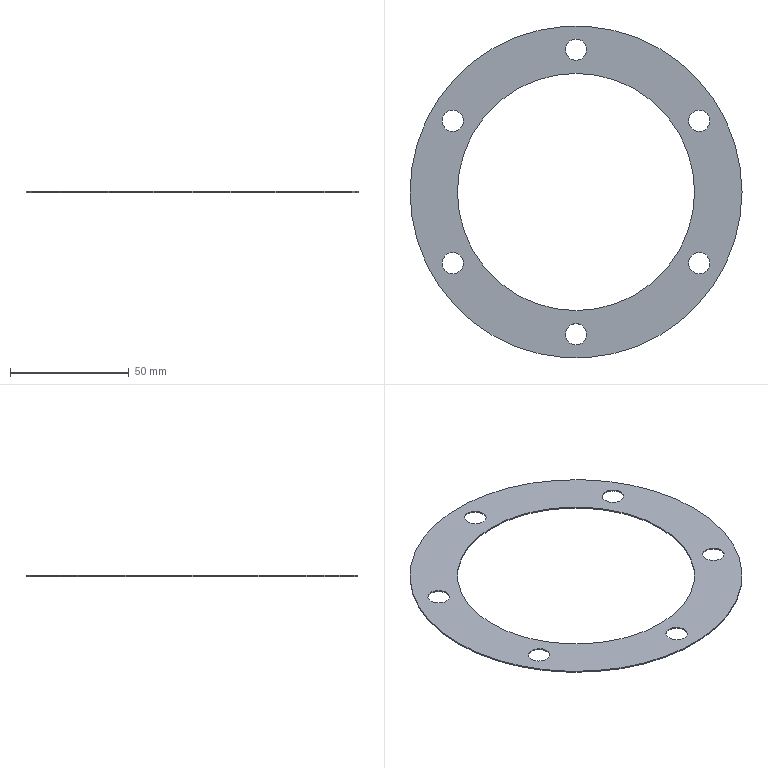Part | SolidWorks | features CirPattern 1, Extrusion 1, ICE 1 | 1 solid | 18 faces | box 140 x 140 x 0.5 mm | volume 3579 mm3 | cylinder 16 | plane 2 | commonest cylinder face diameters 9 x12 100 x2 140 x2
STEP:
#1=CARTESIAN_POINT('',(47.462,30.,0.));
#2=VERTEX_POINT('',#1);
#3=CARTESIAN_POINT('',(56.462,30.,0.));
#4=VERTEX_POINT('',#3);
#5=CARTESIAN_POINT('',(51.962,30.,0.));
#6=DIRECTION('',(0.,0.,1.));
#7=DIRECTION('',(0.5,-0.866,0.));
#8=AXIS2_PLACEMENT_3D('',#5,#6,#7);
#9=CIRCLE('',#8,4.5);
#10=EDGE_CURVE('',#2,#4,#9,.T.);
#11=ORIENTED_EDGE('',*,*,#10,.F.);
#12=CARTESIAN_POINT('',(47.462,30.,0.5));
#13=VERTEX_POINT('',#12);
#14=CARTESIAN_POINT('',(47.462,30.,0.));
#15=DIRECTION('',(0.,0.,1.));
#16=VECTOR('',#15,1000.);
#17=LINE('',#14,#16);
#18=EDGE_CURVE('',#2,#13,#17,.T.);
#19=ORIENTED_EDGE('',*,*,#18,.T.);
#20=CARTESIAN_POINT('',(56.462,30.,0.5));
#21=VERTEX_POINT('',#20);
#22=CARTESIAN_POINT('',(51.962,30.,0.5));
#23=DIRECTION('',(0.,0.,1.));
#24=DIRECTION('',(0.5,-0.866,0.));
#25=AXIS2_PLACEMENT_3D('',#22,#23,#24);
#26=CIRCLE('',#25,4.5);
#27=EDGE_CURVE('',#13,#21,#26,.T.);
#28=ORIENTED_EDGE('',*,*,#27,.T.);
#29=CARTESIAN_POINT('',(56.462,30.,0.));
#30=DIRECTION('',(0.,0.,1.));
#31=VECTOR('',#30,1000.);
#32=LINE('',#29,#31);
#33=EDGE_CURVE('',#4,#21,#32,.T.);
#34=ORIENTED_EDGE('',*,*,#33,.F.);
#35=EDGE_LOOP('',(#11,#19,#28,#34));
#36=FACE_OUTER_BOUND('',#35,.T.);
#37=CARTESIAN_POINT('',(51.962,30.,0.));
#38=DIRECTION('',(0.,0.,1.));
#39=DIRECTION('',(1.,0.,0.));
#40=AXIS2_PLACEMENT_3D('',#37,#38,#39);
#41=CYLINDRICAL_SURFACE('',#40,4.5);
#42=ADVANCED_FACE('',(#36),#41,.F.);
#43=CARTESIAN_POINT('',(47.462,-30.,0.));
#44=VERTEX_POINT('',#43);
#45=CARTESIAN_POINT('',(56.462,-30.,0.));
#46=VERTEX_POINT('',#45);
#47=CARTESIAN_POINT('',(51.962,-30.,0.));
#48=DIRECTION('',(0.,0.,1.));
#49=DIRECTION('',(-0.5,-0.866,0.));
#50=AXIS2_PLACEMENT_3D('',#47,#48,#49);
#51=CIRCLE('',#50,4.5);
#52=EDGE_CURVE('',#44,#46,#51,.T.);
#53=ORIENTED_EDGE('',*,*,#52,.F.);
#54=CARTESIAN_POINT('',(47.462,-30.,0.5));
#55=VERTEX_POINT('',#54);
#56=CARTESIAN_POINT('',(47.462,-30.,0.));
#57=DIRECTION('',(0.,0.,1.));
#58=VECTOR('',#57,1000.);
#59=LINE('',#56,#58);
#60=EDGE_CURVE('',#44,#55,#59,.T.);
#61=ORIENTED_EDGE('',*,*,#60,.T.);
#62=CARTESIAN_POINT('',(56.462,-30.,0.5));
#63=VERTEX_POINT('',#62);
#64=CARTESIAN_POINT('',(51.962,-30.,0.5));
#65=DIRECTION('',(0.,0.,1.));
#66=DIRECTION('',(-0.5,-0.866,0.));
#67=AXIS2_PLACEMENT_3D('',#64,#65,#66);
#68=CIRCLE('',#67,4.5);
#69=EDGE_CURVE('',#55,#63,#68,.T.);
#70=ORIENTED_EDGE('',*,*,#69,.T.);
#71=CARTESIAN_POINT('',(56.462,-30.,0.));
#72=DIRECTION('',(0.,0.,1.));
#73=VECTOR('',#72,1000.);
#74=LINE('',#71,#73);
#75=EDGE_CURVE('',#46,#63,#74,.T.);
#76=ORIENTED_EDGE('',*,*,#75,.F.);
#77=EDGE_LOOP('',(#53,#61,#70,#76));
#78=FACE_OUTER_BOUND('',#77,.T.);
#79=CARTESIAN_POINT('',(51.962,-30.,0.));
#80=DIRECTION('',(0.,0.,1.));
#81=DIRECTION('',(1.,0.,0.));
#82=AXIS2_PLACEMENT_3D('',#79,#80,#81);
#83=CYLINDRICAL_SURFACE('',#82,4.5);
#84=ADVANCED_FACE('',(#78),#83,.F.);
#85=CARTESIAN_POINT('',(-4.5,-60.,0.));
#86=VERTEX_POINT('',#85);
#87=CARTESIAN_POINT('',(4.5,-60.,0.));
#88=VERTEX_POINT('',#87);
#89=CARTESIAN_POINT('',(0.,-60.,0.));
#90=DIRECTION('',(0.,0.,1.));
#91=DIRECTION('',(-1.,0.,0.));
#92=AXIS2_PLACEMENT_3D('',#89,#90,#91);
#93=CIRCLE('',#92,4.5);
#94=EDGE_CURVE('',#86,#88,#93,.T.);
#95=ORIENTED_EDGE('',*,*,#94,.F.);
#96=CARTESIAN_POINT('',(-4.5,-60.,0.5));
#97=VERTEX_POINT('',#96);
#98=CARTESIAN_POINT('',(-4.5,-60.,0.));
#99=DIRECTION('',(0.,0.,1.));
#100=VECTOR('',#99,1000.);
#101=LINE('',#98,#100);
#102=EDGE_CURVE('',#86,#97,#101,.T.);
#103=ORIENTED_EDGE('',*,*,#102,.T.);
#104=CARTESIAN_POINT('',(4.5,-60.,0.5));
#105=VERTEX_POINT('',#104);
#106=CARTESIAN_POINT('',(0.,-60.,0.5));
#107=DIRECTION('',(0.,0.,1.));
#108=DIRECTION('',(-1.,0.,0.));
#109=AXIS2_PLACEMENT_3D('',#106,#107,#108);
#110=CIRCLE('',#109,4.5);
#111=EDGE_CURVE('',#97,#105,#110,.T.);
#112=ORIENTED_EDGE('',*,*,#111,.T.);
#113=CARTESIAN_POINT('',(4.5,-60.,0.));
#114=DIRECTION('',(0.,0.,1.));
#115=VECTOR('',#114,1000.);
#116=LINE('',#113,#115);
#117=EDGE_CURVE('',#88,#105,#116,.T.);
#118=ORIENTED_EDGE('',*,*,#117,.F.);
#119=EDGE_LOOP('',(#95,#103,#112,#118));
#120=FACE_OUTER_BOUND('',#119,.T.);
#121=CARTESIAN_POINT('',(0.,-60.,0.));
#122=DIRECTION('',(0.,0.,1.));
#123=DIRECTION('',(1.,0.,0.));
#124=AXIS2_PLACEMENT_3D('',#121,#122,#123);
#125=CYLINDRICAL_SURFACE('',#124,4.5);
#126=ADVANCED_FACE('',(#120),#125,.F.);
#127=CARTESIAN_POINT('',(-56.462,-30.,0.));
#128=VERTEX_POINT('',#127);
#129=CARTESIAN_POINT('',(-47.462,-30.,0.));
#130=VERTEX_POINT('',#129);
#131=CARTESIAN_POINT('',(-51.962,-30.,0.));
#132=DIRECTION('',(0.,0.,1.));
#133=DIRECTION('',(-0.5,0.866,0.));
#134=AXIS2_PLACEMENT_3D('',#131,#132,#133);
#135=CIRCLE('',#134,4.5);
#136=EDGE_CURVE('',#128,#130,#135,.T.);
#137=ORIENTED_EDGE('',*,*,#136,.F.);
#138=CARTESIAN_POINT('',(-56.462,-30.,0.5));
#139=VERTEX_POINT('',#138);
#140=CARTESIAN_POINT('',(-56.462,-30.,0.));
#141=DIRECTION('',(0.,0.,1.));
#142=VECTOR('',#141,1000.);
#143=LINE('',#140,#142);
#144=EDGE_CURVE('',#128,#139,#143,.T.);
#145=ORIENTED_EDGE('',*,*,#144,.T.);
#146=CARTESIAN_POINT('',(-47.462,-30.,0.5));
#147=VERTEX_POINT('',#146);
#148=CARTESIAN_POINT('',(-51.962,-30.,0.5));
#149=DIRECTION('',(0.,0.,1.));
#150=DIRECTION('',(-0.5,0.866,0.));
#151=AXIS2_PLACEMENT_3D('',#148,#149,#150);
#152=CIRCLE('',#151,4.5);
#153=EDGE_CURVE('',#139,#147,#152,.T.);
#154=ORIENTED_EDGE('',*,*,#153,.T.);
#155=CARTESIAN_POINT('',(-47.462,-30.,0.));
#156=DIRECTION('',(0.,0.,1.));
#157=VECTOR('',#156,1000.);
#158=LINE('',#155,#157);
#159=EDGE_CURVE('',#130,#147,#158,.T.);
#160=ORIENTED_EDGE('',*,*,#159,.F.);
#161=EDGE_LOOP('',(#137,#145,#154,#160));
#162=FACE_OUTER_BOUND('',#161,.T.);
#163=CARTESIAN_POINT('',(-51.962,-30.,0.));
#164=DIRECTION('',(0.,0.,1.));
#165=DIRECTION('',(1.,0.,0.));
#166=AXIS2_PLACEMENT_3D('',#163,#164,#165);
#167=CYLINDRICAL_SURFACE('',#166,4.5);
#168=ADVANCED_FACE('',(#162),#167,.F.);
#169=CARTESIAN_POINT('',(-56.462,30.,0.));
#170=VERTEX_POINT('',#169);
#171=CARTESIAN_POINT('',(-47.462,30.,0.));
#172=VERTEX_POINT('',#171);
#173=CARTESIAN_POINT('',(-51.962,30.,0.));
#174=DIRECTION('',(0.,0.,1.));
#175=DIRECTION('',(0.5,0.866,0.));
#176=AXIS2_PLACEMENT_3D('',#173,#174,#175);
#177=CIRCLE('',#176,4.5);
#178=EDGE_CURVE('',#170,#172,#177,.T.);
#179=ORIENTED_EDGE('',*,*,#178,.F.);
#180=CARTESIAN_POINT('',(-56.462,30.,0.5));
#181=VERTEX_POINT('',#180);
#182=CARTESIAN_POINT('',(-56.462,30.,0.));
#183=DIRECTION('',(0.,0.,1.));
#184=VECTOR('',#183,1000.);
#185=LINE('',#182,#184);
#186=EDGE_CURVE('',#170,#181,#185,.T.);
#187=ORIENTED_EDGE('',*,*,#186,.T.);
#188=CARTESIAN_POINT('',(-47.462,30.,0.5));
#189=VERTEX_POINT('',#188);
#190=CARTESIAN_POINT('',(-51.962,30.,0.5));
#191=DIRECTION('',(0.,0.,1.));
#192=DIRECTION('',(0.5,0.866,0.));
#193=AXIS2_PLACEMENT_3D('',#190,#191,#192);
#194=CIRCLE('',#193,4.5);
#195=EDGE_CURVE('',#181,#189,#194,.T.);
#196=ORIENTED_EDGE('',*,*,#195,.T.);
#197=CARTESIAN_POINT('',(-47.462,30.,0.));
#198=DIRECTION('',(0.,0.,1.));
#199=VECTOR('',#198,1000.);
#200=LINE('',#197,#199);
#201=EDGE_CURVE('',#172,#189,#200,.T.);
#202=ORIENTED_EDGE('',*,*,#201,.F.);
#203=EDGE_LOOP('',(#179,#187,#196,#202));
#204=FACE_OUTER_BOUND('',#203,.T.);
#205=CARTESIAN_POINT('',(-51.962,30.,0.));
#206=DIRECTION('',(0.,0.,1.));
#207=DIRECTION('',(1.,0.,0.));
#208=AXIS2_PLACEMENT_3D('',#205,#206,#207);
#209=CYLINDRICAL_SURFACE('',#208,4.5);
#210=ADVANCED_FACE('',(#204),#209,.F.);
#211=CARTESIAN_POINT('',(-4.5,60.,0.));
#212=VERTEX_POINT('',#211);
#213=CARTESIAN_POINT('',(4.5,60.,0.));
#214=VERTEX_POINT('',#213);
#215=CARTESIAN_POINT('',(0.,60.,0.));
#216=DIRECTION('',(0.,0.,1.));
#217=DIRECTION('',(1.,0.,0.));
#218=AXIS2_PLACEMENT_3D('',#215,#216,#217);
#219=CIRCLE('',#218,4.5);
#220=EDGE_CURVE('',#212,#214,#219,.T.);
#221=ORIENTED_EDGE('',*,*,#220,.F.);
#222=CARTESIAN_POINT('',(-4.5,60.,0.5));
#223=VERTEX_POINT('',#222);
#224=CARTESIAN_POINT('',(-4.5,60.,0.));
#225=DIRECTION('',(0.,0.,1.));
#226=VECTOR('',#225,1000.);
#227=LINE('',#224,#226);
#228=EDGE_CURVE('',#212,#223,#227,.T.);
#229=ORIENTED_EDGE('',*,*,#228,.T.);
#230=CARTESIAN_POINT('',(4.5,60.,0.5));
#231=VERTEX_POINT('',#230);
#232=CARTESIAN_POINT('',(0.,60.,0.5));
#233=DIRECTION('',(0.,0.,1.));
#234=DIRECTION('',(1.,0.,0.));
#235=AXIS2_PLACEMENT_3D('',#232,#233,#234);
#236=CIRCLE('',#235,4.5);
#237=EDGE_CURVE('',#223,#231,#236,.T.);
#238=ORIENTED_EDGE('',*,*,#237,.T.);
#239=CARTESIAN_POINT('',(4.5,60.,0.));
#240=DIRECTION('',(0.,0.,1.));
#241=VECTOR('',#240,1000.);
#242=LINE('',#239,#241);
#243=EDGE_CURVE('',#214,#231,#242,.T.);
#244=ORIENTED_EDGE('',*,*,#243,.F.);
#245=EDGE_LOOP('',(#221,#229,#238,#244));
#246=FACE_OUTER_BOUND('',#245,.T.);
#247=CARTESIAN_POINT('',(0.,60.,0.));
#248=DIRECTION('',(0.,0.,1.));
#249=DIRECTION('',(1.,0.,0.));
#250=AXIS2_PLACEMENT_3D('',#247,#248,#249);
#251=CYLINDRICAL_SURFACE('',#250,4.5);
#252=ADVANCED_FACE('',(#246),#251,.F.);
#253=CARTESIAN_POINT('',(-50.,0.,0.5));
#254=VERTEX_POINT('',#253);
#255=CARTESIAN_POINT('',(50.,0.,0.5));
#256=VERTEX_POINT('',#255);
#257=CARTESIAN_POINT('',(0.,0.,0.5));
#258=DIRECTION('',(0.,0.,1.));
#259=DIRECTION('',(1.,0.,0.));
#260=AXIS2_PLACEMENT_3D('',#257,#258,#259);
#261=CIRCLE('',#260,50.);
#262=EDGE_CURVE('',#254,#256,#261,.T.);
#263=ORIENTED_EDGE('',*,*,#262,.T.);
#264=CARTESIAN_POINT('',(50.,0.,0.));
#265=VERTEX_POINT('',#264);
#266=CARTESIAN_POINT('',(50.,0.,0.5));
#267=DIRECTION('',(0.,0.,-1.));
#268=VECTOR('',#267,1000.);
#269=LINE('',#266,#268);
#270=EDGE_CURVE('',#256,#265,#269,.T.);
#271=ORIENTED_EDGE('',*,*,#270,.T.);
#272=CARTESIAN_POINT('',(-50.,0.,0.));
#273=VERTEX_POINT('',#272);
#274=CARTESIAN_POINT('',(0.,0.,0.));
#275=DIRECTION('',(0.,0.,1.));
#276=DIRECTION('',(1.,0.,0.));
#277=AXIS2_PLACEMENT_3D('',#274,#275,#276);
#278=CIRCLE('',#277,50.);
#279=EDGE_CURVE('',#273,#265,#278,.T.);
#280=ORIENTED_EDGE('',*,*,#279,.F.);
#281=CARTESIAN_POINT('',(-50.,0.,0.5));
#282=DIRECTION('',(0.,0.,-1.));
#283=VECTOR('',#282,1000.);
#284=LINE('',#281,#283);
#285=EDGE_CURVE('',#254,#273,#284,.T.);
#286=ORIENTED_EDGE('',*,*,#285,.F.);
#287=EDGE_LOOP('',(#263,#271,#280,#286));
#288=FACE_OUTER_BOUND('',#287,.T.);
#289=CARTESIAN_POINT('',(0.,0.,0.5));
#290=DIRECTION('',(0.,0.,-1.));
#291=DIRECTION('',(-1.,0.,0.));
#292=AXIS2_PLACEMENT_3D('',#289,#290,#291);
#293=CYLINDRICAL_SURFACE('',#292,50.);
#294=ADVANCED_FACE('',(#288),#293,.F.);
#295=CARTESIAN_POINT('',(70.,0.,0.5));
#296=VERTEX_POINT('',#295);
#297=CARTESIAN_POINT('',(-70.,0.,0.5));
#298=VERTEX_POINT('',#297);
#299=CARTESIAN_POINT('',(0.,0.,0.5));
#300=DIRECTION('',(0.,0.,1.));
#301=DIRECTION('',(1.,0.,0.));
#302=AXIS2_PLACEMENT_3D('',#299,#300,#301);
#303=CIRCLE('',#302,70.);
#304=EDGE_CURVE('',#296,#298,#303,.T.);
#305=ORIENTED_EDGE('',*,*,#304,.F.);
#306=CARTESIAN_POINT('',(70.,0.,0.));
#307=VERTEX_POINT('',#306);
#308=CARTESIAN_POINT('',(70.,0.,0.5));
#309=DIRECTION('',(0.,0.,-1.));
#310=VECTOR('',#309,1000.);
#311=LINE('',#308,#310);
#312=EDGE_CURVE('',#296,#307,#311,.T.);
#313=ORIENTED_EDGE('',*,*,#312,.T.);
#314=CARTESIAN_POINT('',(-70.,0.,0.));
#315=VERTEX_POINT('',#314);
#316=CARTESIAN_POINT('',(0.,0.,0.));
#317=DIRECTION('',(0.,0.,1.));
#318=DIRECTION('',(1.,0.,0.));
#319=AXIS2_PLACEMENT_3D('',#316,#317,#318);
#320=CIRCLE('',#319,70.);
#321=EDGE_CURVE('',#307,#315,#320,.T.);
#322=ORIENTED_EDGE('',*,*,#321,.T.);
#323=CARTESIAN_POINT('',(-70.,0.,0.5));
#324=DIRECTION('',(0.,0.,-1.));
#325=VECTOR('',#324,1000.);
#326=LINE('',#323,#325);
#327=EDGE_CURVE('',#298,#315,#326,.T.);
#328=ORIENTED_EDGE('',*,*,#327,.F.);
#329=EDGE_LOOP('',(#305,#313,#322,#328));
#330=FACE_OUTER_BOUND('',#329,.T.);
#331=CARTESIAN_POINT('',(0.,0.,0.5));
#332=DIRECTION('',(0.,0.,-1.));
#333=DIRECTION('',(-1.,0.,0.));
#334=AXIS2_PLACEMENT_3D('',#331,#332,#333);
#335=CYLINDRICAL_SURFACE('',#334,70.);
#336=ADVANCED_FACE('',(#330),#335,.T.);
#337=CARTESIAN_POINT('',(51.962,30.,0.5));
#338=DIRECTION('',(0.,0.,1.));
#339=DIRECTION('',(0.5,-0.866,0.));
#340=AXIS2_PLACEMENT_3D('',#337,#338,#339);
#341=CIRCLE('',#340,4.5);
#342=EDGE_CURVE('',#21,#13,#341,.T.);
#343=ORIENTED_EDGE('',*,*,#342,.F.);
#344=ORIENTED_EDGE('',*,*,#27,.F.);
#345=EDGE_LOOP('',(#343,#344));
#346=FACE_BOUND('',#345,.T.);
#347=CARTESIAN_POINT('',(51.962,-30.,0.5));
#348=DIRECTION('',(0.,0.,1.));
#349=DIRECTION('',(-0.5,-0.866,0.));
#350=AXIS2_PLACEMENT_3D('',#347,#348,#349);
#351=CIRCLE('',#350,4.5);
#352=EDGE_CURVE('',#63,#55,#351,.T.);
#353=ORIENTED_EDGE('',*,*,#352,.F.);
#354=ORIENTED_EDGE('',*,*,#69,.F.);
#355=EDGE_LOOP('',(#353,#354));
#356=FACE_BOUND('',#355,.T.);
#357=CARTESIAN_POINT('',(0.,-60.,0.5));
#358=DIRECTION('',(0.,0.,1.));
#359=DIRECTION('',(-1.,0.,0.));
#360=AXIS2_PLACEMENT_3D('',#357,#358,#359);
#361=CIRCLE('',#360,4.5);
#362=EDGE_CURVE('',#105,#97,#361,.T.);
#363=ORIENTED_EDGE('',*,*,#362,.F.);
#364=ORIENTED_EDGE('',*,*,#111,.F.);
#365=EDGE_LOOP('',(#363,#364));
#366=FACE_BOUND('',#365,.T.);
#367=CARTESIAN_POINT('',(-51.962,-30.,0.5));
#368=DIRECTION('',(0.,0.,1.));
#369=DIRECTION('',(-0.5,0.866,0.));
#370=AXIS2_PLACEMENT_3D('',#367,#368,#369);
#371=CIRCLE('',#370,4.5);
#372=EDGE_CURVE('',#147,#139,#371,.T.);
#373=ORIENTED_EDGE('',*,*,#372,.F.);
#374=ORIENTED_EDGE('',*,*,#153,.F.);
#375=EDGE_LOOP('',(#373,#374));
#376=FACE_BOUND('',#375,.T.);
#377=CARTESIAN_POINT('',(-51.962,30.,0.5));
#378=DIRECTION('',(0.,0.,1.));
#379=DIRECTION('',(0.5,0.866,0.));
#380=AXIS2_PLACEMENT_3D('',#377,#378,#379);
#381=CIRCLE('',#380,4.5);
#382=EDGE_CURVE('',#189,#181,#381,.T.);
#383=ORIENTED_EDGE('',*,*,#382,.F.);
#384=ORIENTED_EDGE('',*,*,#195,.F.);
#385=EDGE_LOOP('',(#383,#384));
#386=FACE_BOUND('',#385,.T.);
#387=CARTESIAN_POINT('',(0.,60.,0.5));
#388=DIRECTION('',(0.,0.,1.));
#389=DIRECTION('',(1.,0.,0.));
#390=AXIS2_PLACEMENT_3D('',#387,#388,#389);
#391=CIRCLE('',#390,4.5);
#392=EDGE_CURVE('',#231,#223,#391,.T.);
#393=ORIENTED_EDGE('',*,*,#392,.F.);
#394=ORIENTED_EDGE('',*,*,#237,.F.);
#395=EDGE_LOOP('',(#393,#394));
#396=FACE_BOUND('',#395,.T.);
#397=CARTESIAN_POINT('',(0.,0.,0.5));
#398=DIRECTION('',(0.,0.,1.));
#399=DIRECTION('',(1.,0.,0.));
#400=AXIS2_PLACEMENT_3D('',#397,#398,#399);
#401=CIRCLE('',#400,70.);
#402=EDGE_CURVE('',#298,#296,#401,.T.);
#403=ORIENTED_EDGE('',*,*,#402,.T.);
#404=ORIENTED_EDGE('',*,*,#304,.T.);
#405=EDGE_LOOP('',(#403,#404));
#406=FACE_OUTER_BOUND('',#405,.T.);
#407=ORIENTED_EDGE('',*,*,#262,.F.);
#408=CARTESIAN_POINT('',(0.,0.,0.5));
#409=DIRECTION('',(0.,0.,1.));
#410=DIRECTION('',(1.,0.,0.));
#411=AXIS2_PLACEMENT_3D('',#408,#409,#410);
#412=CIRCLE('',#411,50.);
#413=EDGE_CURVE('',#256,#254,#412,.T.);
#414=ORIENTED_EDGE('',*,*,#413,.F.);
#415=EDGE_LOOP('',(#407,#414));
#416=FACE_BOUND('',#415,.T.);
#417=CARTESIAN_POINT('',(0.,0.,0.5));
#418=DIRECTION('',(0.,0.,1.));
#419=DIRECTION('',(1.,0.,0.));
#420=AXIS2_PLACEMENT_3D('',#417,#418,#419);
#421=PLANE('',#420);
#422=ADVANCED_FACE('',(#346,#356,#366,#376,#386,#396,#406,#416),#421,.T.);
#423=CARTESIAN_POINT('',(51.962,30.,0.));
#424=DIRECTION('',(0.,0.,1.));
#425=DIRECTION('',(0.5,-0.866,0.));
#426=AXIS2_PLACEMENT_3D('',#423,#424,#425);
#427=CIRCLE('',#426,4.5);
#428=EDGE_CURVE('',#4,#2,#427,.T.);
#429=ORIENTED_EDGE('',*,*,#428,.T.);
#430=ORIENTED_EDGE('',*,*,#10,.T.);
#431=EDGE_LOOP('',(#429,#430));
#432=FACE_BOUND('',#431,.T.);
#433=CARTESIAN_POINT('',(51.962,-30.,0.));
#434=DIRECTION('',(0.,0.,1.));
#435=DIRECTION('',(-0.5,-0.866,0.));
#436=AXIS2_PLACEMENT_3D('',#433,#434,#435);
#437=CIRCLE('',#436,4.5);
#438=EDGE_CURVE('',#46,#44,#437,.T.);
#439=ORIENTED_EDGE('',*,*,#438,.T.);
#440=ORIENTED_EDGE('',*,*,#52,.T.);
#441=EDGE_LOOP('',(#439,#440));
#442=FACE_BOUND('',#441,.T.);
#443=CARTESIAN_POINT('',(0.,-60.,0.));
#444=DIRECTION('',(0.,0.,1.));
#445=DIRECTION('',(-1.,0.,0.));
#446=AXIS2_PLACEMENT_3D('',#443,#444,#445);
#447=CIRCLE('',#446,4.5);
#448=EDGE_CURVE('',#88,#86,#447,.T.);
#449=ORIENTED_EDGE('',*,*,#448,.T.);
#450=ORIENTED_EDGE('',*,*,#94,.T.);
#451=EDGE_LOOP('',(#449,#450));
#452=FACE_BOUND('',#451,.T.);
#453=CARTESIAN_POINT('',(-51.962,-30.,0.));
#454=DIRECTION('',(0.,0.,1.));
#455=DIRECTION('',(-0.5,0.866,0.));
#456=AXIS2_PLACEMENT_3D('',#453,#454,#455);
#457=CIRCLE('',#456,4.5);
#458=EDGE_CURVE('',#130,#128,#457,.T.);
#459=ORIENTED_EDGE('',*,*,#458,.T.);
#460=ORIENTED_EDGE('',*,*,#136,.T.);
#461=EDGE_LOOP('',(#459,#460));
#462=FACE_BOUND('',#461,.T.);
#463=CARTESIAN_POINT('',(-51.962,30.,0.));
#464=DIRECTION('',(0.,0.,1.));
#465=DIRECTION('',(0.5,0.866,0.));
#466=AXIS2_PLACEMENT_3D('',#463,#464,#465);
#467=CIRCLE('',#466,4.5);
#468=EDGE_CURVE('',#172,#170,#467,.T.);
#469=ORIENTED_EDGE('',*,*,#468,.T.);
#470=ORIENTED_EDGE('',*,*,#178,.T.);
#471=EDGE_LOOP('',(#469,#470));
#472=FACE_BOUND('',#471,.T.);
#473=CARTESIAN_POINT('',(0.,60.,0.));
#474=DIRECTION('',(0.,0.,1.));
#475=DIRECTION('',(1.,0.,0.));
#476=AXIS2_PLACEMENT_3D('',#473,#474,#475);
#477=CIRCLE('',#476,4.5);
#478=EDGE_CURVE('',#214,#212,#477,.T.);
#479=ORIENTED_EDGE('',*,*,#478,.T.);
#480=ORIENTED_EDGE('',*,*,#220,.T.);
#481=EDGE_LOOP('',(#479,#480));
#482=FACE_BOUND('',#481,.T.);
#483=CARTESIAN_POINT('',(0.,0.,0.));
#484=DIRECTION('',(0.,0.,1.));
#485=DIRECTION('',(1.,0.,0.));
#486=AXIS2_PLACEMENT_3D('',#483,#484,#485);
#487=CIRCLE('',#486,70.);
#488=EDGE_CURVE('',#315,#307,#487,.T.);
#489=ORIENTED_EDGE('',*,*,#488,.F.);
#490=ORIENTED_EDGE('',*,*,#321,.F.);
#491=EDGE_LOOP('',(#489,#490));
#492=FACE_OUTER_BOUND('',#491,.T.);
#493=ORIENTED_EDGE('',*,*,#279,.T.);
#494=CARTESIAN_POINT('',(0.,0.,0.));
#495=DIRECTION('',(0.,0.,1.));
#496=DIRECTION('',(1.,0.,0.));
#497=AXIS2_PLACEMENT_3D('',#494,#495,#496);
#498=CIRCLE('',#497,50.);
#499=EDGE_CURVE('',#265,#273,#498,.T.);
#500=ORIENTED_EDGE('',*,*,#499,.T.);
#501=EDGE_LOOP('',(#493,#500));
#502=FACE_BOUND('',#501,.T.);
#503=CARTESIAN_POINT('',(0.,0.,0.));
#504=DIRECTION('',(0.,0.,1.));
#505=DIRECTION('',(1.,0.,0.));
#506=AXIS2_PLACEMENT_3D('',#503,#504,#505);
#507=PLANE('',#506);
#508=ADVANCED_FACE('',(#432,#442,#452,#462,#472,#482,#492,#502),#507,.F.);
#509=ORIENTED_EDGE('',*,*,#312,.F.);
#510=ORIENTED_EDGE('',*,*,#402,.F.);
#511=ORIENTED_EDGE('',*,*,#327,.T.);
#512=ORIENTED_EDGE('',*,*,#488,.T.);
#513=EDGE_LOOP('',(#509,#510,#511,#512));
#514=FACE_OUTER_BOUND('',#513,.T.);
#515=CARTESIAN_POINT('',(0.,0.,0.5));
#516=DIRECTION('',(0.,0.,-1.));
#517=DIRECTION('',(-1.,0.,0.));
#518=AXIS2_PLACEMENT_3D('',#515,#516,#517);
#519=CYLINDRICAL_SURFACE('',#518,70.);
#520=ADVANCED_FACE('',(#514),#519,.T.);
#521=ORIENTED_EDGE('',*,*,#270,.F.);
#522=ORIENTED_EDGE('',*,*,#413,.T.);
#523=ORIENTED_EDGE('',*,*,#285,.T.);
#524=ORIENTED_EDGE('',*,*,#499,.F.);
#525=EDGE_LOOP('',(#521,#522,#523,#524));
#526=FACE_OUTER_BOUND('',#525,.T.);
#527=CARTESIAN_POINT('',(0.,0.,0.5));
#528=DIRECTION('',(0.,0.,-1.));
#529=DIRECTION('',(-1.,0.,0.));
#530=AXIS2_PLACEMENT_3D('',#527,#528,#529);
#531=CYLINDRICAL_SURFACE('',#530,50.);
#532=ADVANCED_FACE('',(#526),#531,.F.);
#533=ORIENTED_EDGE('',*,*,#228,.F.);
#534=ORIENTED_EDGE('',*,*,#478,.F.);
#535=ORIENTED_EDGE('',*,*,#243,.T.);
#536=ORIENTED_EDGE('',*,*,#392,.T.);
#537=EDGE_LOOP('',(#533,#534,#535,#536));
#538=FACE_OUTER_BOUND('',#537,.T.);
#539=CARTESIAN_POINT('',(0.,60.,0.));
#540=DIRECTION('',(0.,0.,1.));
#541=DIRECTION('',(1.,0.,0.));
#542=AXIS2_PLACEMENT_3D('',#539,#540,#541);
#543=CYLINDRICAL_SURFACE('',#542,4.5);
#544=ADVANCED_FACE('',(#538),#543,.F.);
#545=ORIENTED_EDGE('',*,*,#186,.F.);
#546=ORIENTED_EDGE('',*,*,#468,.F.);
#547=ORIENTED_EDGE('',*,*,#201,.T.);
#548=ORIENTED_EDGE('',*,*,#382,.T.);
#549=EDGE_LOOP('',(#545,#546,#547,#548));
#550=FACE_OUTER_BOUND('',#549,.T.);
#551=CARTESIAN_POINT('',(-51.962,30.,0.));
#552=DIRECTION('',(0.,0.,1.));
#553=DIRECTION('',(1.,0.,0.));
#554=AXIS2_PLACEMENT_3D('',#551,#552,#553);
#555=CYLINDRICAL_SURFACE('',#554,4.5);
#556=ADVANCED_FACE('',(#550),#555,.F.);
#557=ORIENTED_EDGE('',*,*,#144,.F.);
#558=ORIENTED_EDGE('',*,*,#458,.F.);
#559=ORIENTED_EDGE('',*,*,#159,.T.);
#560=ORIENTED_EDGE('',*,*,#372,.T.);
#561=EDGE_LOOP('',(#557,#558,#559,#560));
#562=FACE_OUTER_BOUND('',#561,.T.);
#563=CARTESIAN_POINT('',(-51.962,-30.,0.));
#564=DIRECTION('',(0.,0.,1.));
#565=DIRECTION('',(1.,0.,0.));
#566=AXIS2_PLACEMENT_3D('',#563,#564,#565);
#567=CYLINDRICAL_SURFACE('',#566,4.5);
#568=ADVANCED_FACE('',(#562),#567,.F.);
#569=ORIENTED_EDGE('',*,*,#102,.F.);
#570=ORIENTED_EDGE('',*,*,#448,.F.);
#571=ORIENTED_EDGE('',*,*,#117,.T.);
#572=ORIENTED_EDGE('',*,*,#362,.T.);
#573=EDGE_LOOP('',(#569,#570,#571,#572));
#574=FACE_OUTER_BOUND('',#573,.T.);
#575=CARTESIAN_POINT('',(0.,-60.,0.));
#576=DIRECTION('',(0.,0.,1.));
#577=DIRECTION('',(1.,0.,0.));
#578=AXIS2_PLACEMENT_3D('',#575,#576,#577);
#579=CYLINDRICAL_SURFACE('',#578,4.5);
#580=ADVANCED_FACE('',(#574),#579,.F.);
#581=ORIENTED_EDGE('',*,*,#60,.F.);
#582=ORIENTED_EDGE('',*,*,#438,.F.);
#583=ORIENTED_EDGE('',*,*,#75,.T.);
#584=ORIENTED_EDGE('',*,*,#352,.T.);
#585=EDGE_LOOP('',(#581,#582,#583,#584));
#586=FACE_OUTER_BOUND('',#585,.T.);
#587=CARTESIAN_POINT('',(51.962,-30.,0.));
#588=DIRECTION('',(0.,0.,1.));
#589=DIRECTION('',(1.,0.,0.));
#590=AXIS2_PLACEMENT_3D('',#587,#588,#589);
#591=CYLINDRICAL_SURFACE('',#590,4.5);
#592=ADVANCED_FACE('',(#586),#591,.F.);
#593=ORIENTED_EDGE('',*,*,#18,.F.);
#594=ORIENTED_EDGE('',*,*,#428,.F.);
#595=ORIENTED_EDGE('',*,*,#33,.T.);
#596=ORIENTED_EDGE('',*,*,#342,.T.);
#597=EDGE_LOOP('',(#593,#594,#595,#596));
#598=FACE_OUTER_BOUND('',#597,.T.);
#599=CARTESIAN_POINT('',(51.962,30.,0.));
#600=DIRECTION('',(0.,0.,1.));
#601=DIRECTION('',(1.,0.,0.));
#602=AXIS2_PLACEMENT_3D('',#599,#600,#601);
#603=CYLINDRICAL_SURFACE('',#602,4.5);
#604=ADVANCED_FACE('',(#598),#603,.F.);
#605=CLOSED_SHELL('',(#42,#84,#126,#168,#210,#252,#294,#336,#422,#508,#520,#532,#544,#556,#568,#580,#592,#604));
#606=MANIFOLD_SOLID_BREP('',#605);
#607=CARTESIAN_POINT('',(0.,0.,0.));
#608=DIRECTION('',(0.,0.,1.));
#609=DIRECTION('',(1.,0.,0.));
#610=AXIS2_PLACEMENT_3D('',#607,#608,#609);
#611=(LENGTH_UNIT()NAMED_UNIT(*)SI_UNIT(.MILLI.,.METRE.));
#612=UNCERTAINTY_MEASURE_WITH_UNIT(LENGTH_MEASURE(0.00001),#611,'','');
#613=(NAMED_UNIT(*)PLANE_ANGLE_UNIT()SI_UNIT($,.RADIAN.));
#614=(NAMED_UNIT(*)SI_UNIT($,.STERADIAN.)SOLID_ANGLE_UNIT());
#615=(GEOMETRIC_REPRESENTATION_CONTEXT(3)GLOBAL_UNCERTAINTY_ASSIGNED_CONTEXT((#612))GLOBAL_UNIT_ASSIGNED_CONTEXT((#611,#613,#614))REPRESENTATION_CONTEXT('',''));
#616=ADVANCED_BREP_SHAPE_REPRESENTATION('',(#606,#610),#615);